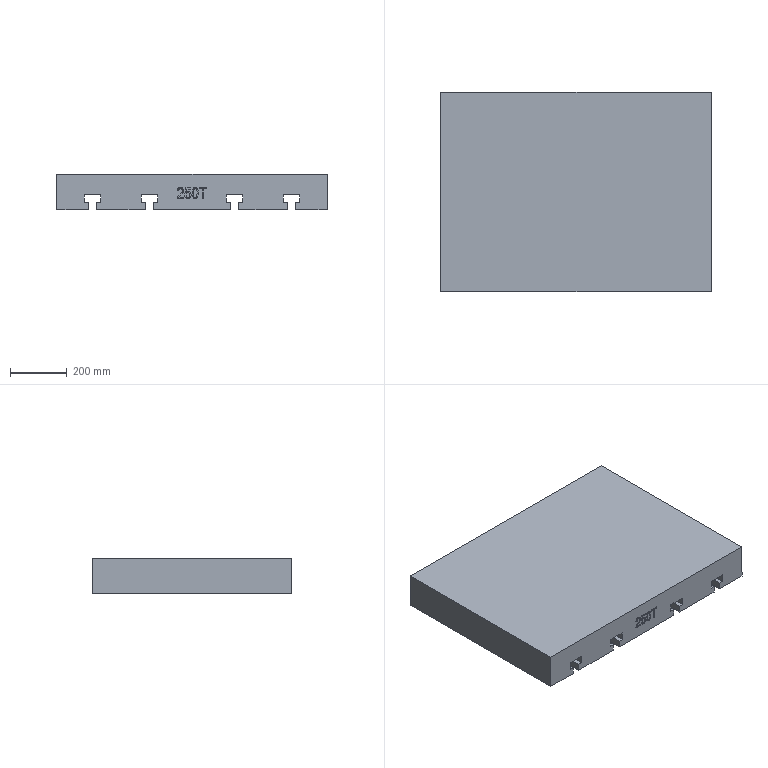Part | NX | features LIN_SOLID_COLOR 2 | 1 solid | 89 faces | box 950 x 700 x 125 mm | volume 76616379 mm3 | plane 62 | spline 27